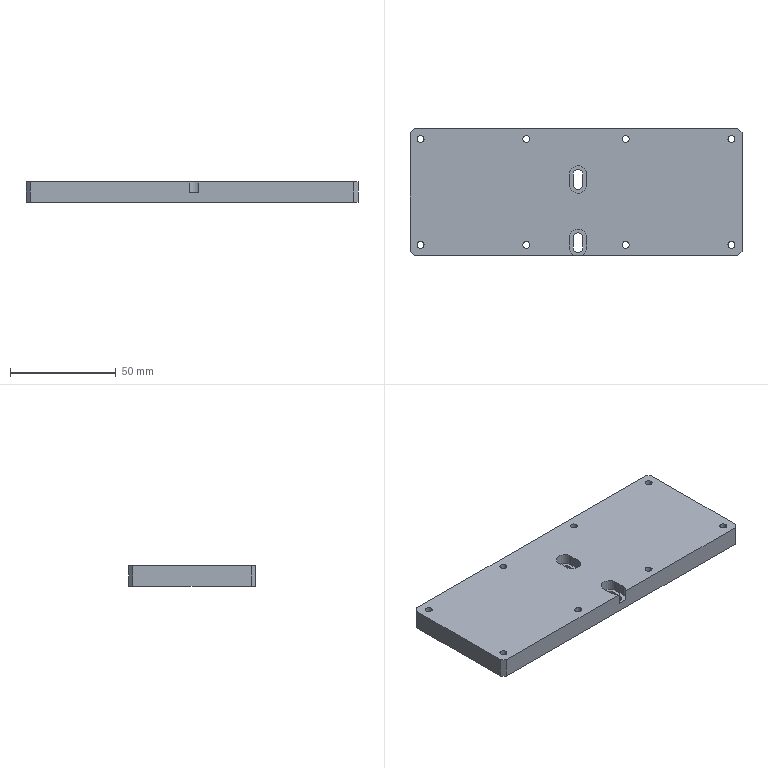Part | STEP file | 05-02-02 adjustment platform base plate | 1 solid | 45 faces | box 157 x 60 x 9.5 mm | volume 87518 mm3 | cylinder 25 | plane 20 | commonest cylinder face diameters 3.3 x16 8 x5 4.5 x4
STEP:
#1=CARTESIAN_POINT('',(71.85,25.,0.));
#2=VERTEX_POINT('',#1);
#3=CARTESIAN_POINT('',(75.15,25.,0.));
#4=VERTEX_POINT('',#3);
#5=CARTESIAN_POINT('',(73.5,25.,0.));
#6=DIRECTION('',(0.,0.,1.));
#7=DIRECTION('',(1.,0.,0.));
#8=AXIS2_PLACEMENT_3D('',#5,#6,#7);
#9=CIRCLE('',#8,1.65);
#10=EDGE_CURVE('',#2,#4,#9,.T.);
#11=ORIENTED_EDGE('',*,*,#10,.F.);
#12=CARTESIAN_POINT('',(71.85,25.,9.5));
#13=VERTEX_POINT('',#12);
#14=CARTESIAN_POINT('',(71.85,25.,9.5));
#15=DIRECTION('',(0.,0.,1.));
#16=VECTOR('',#15,1000.);
#17=LINE('',#14,#16);
#18=EDGE_CURVE('',#2,#13,#17,.T.);
#19=ORIENTED_EDGE('',*,*,#18,.T.);
#20=CARTESIAN_POINT('',(75.15,25.,9.5));
#21=VERTEX_POINT('',#20);
#22=CARTESIAN_POINT('',(73.5,25.,9.5));
#23=DIRECTION('',(0.,0.,1.));
#24=DIRECTION('',(1.,0.,0.));
#25=AXIS2_PLACEMENT_3D('',#22,#23,#24);
#26=CIRCLE('',#25,1.65);
#27=EDGE_CURVE('',#13,#21,#26,.T.);
#28=ORIENTED_EDGE('',*,*,#27,.T.);
#29=CARTESIAN_POINT('',(75.15,25.,9.5));
#30=DIRECTION('',(0.,0.,1.));
#31=VECTOR('',#30,1000.);
#32=LINE('',#29,#31);
#33=EDGE_CURVE('',#4,#21,#32,.T.);
#34=ORIENTED_EDGE('',*,*,#33,.F.);
#35=EDGE_LOOP('',(#11,#19,#28,#34));
#36=FACE_OUTER_BOUND('',#35,.T.);
#37=CARTESIAN_POINT('',(73.5,25.,9.5));
#38=DIRECTION('',(0.,0.,1.));
#39=DIRECTION('',(1.,0.,0.));
#40=AXIS2_PLACEMENT_3D('',#37,#38,#39);
#41=CYLINDRICAL_SURFACE('',#40,1.65);
#42=ADVANCED_FACE('',(#36),#41,.F.);
#43=CARTESIAN_POINT('',(21.85,-25.,0.));
#44=VERTEX_POINT('',#43);
#45=CARTESIAN_POINT('',(25.15,-25.,0.));
#46=VERTEX_POINT('',#45);
#47=CARTESIAN_POINT('',(23.5,-25.,0.));
#48=DIRECTION('',(0.,0.,1.));
#49=DIRECTION('',(1.,0.,0.));
#50=AXIS2_PLACEMENT_3D('',#47,#48,#49);
#51=CIRCLE('',#50,1.65);
#52=EDGE_CURVE('',#44,#46,#51,.T.);
#53=ORIENTED_EDGE('',*,*,#52,.F.);
#54=CARTESIAN_POINT('',(21.85,-25.,9.5));
#55=VERTEX_POINT('',#54);
#56=CARTESIAN_POINT('',(21.85,-25.,9.5));
#57=DIRECTION('',(0.,0.,1.));
#58=VECTOR('',#57,1000.);
#59=LINE('',#56,#58);
#60=EDGE_CURVE('',#44,#55,#59,.T.);
#61=ORIENTED_EDGE('',*,*,#60,.T.);
#62=CARTESIAN_POINT('',(25.15,-25.,9.5));
#63=VERTEX_POINT('',#62);
#64=CARTESIAN_POINT('',(23.5,-25.,9.5));
#65=DIRECTION('',(0.,0.,1.));
#66=DIRECTION('',(1.,0.,0.));
#67=AXIS2_PLACEMENT_3D('',#64,#65,#66);
#68=CIRCLE('',#67,1.65);
#69=EDGE_CURVE('',#55,#63,#68,.T.);
#70=ORIENTED_EDGE('',*,*,#69,.T.);
#71=CARTESIAN_POINT('',(25.15,-25.,9.5));
#72=DIRECTION('',(0.,0.,1.));
#73=VECTOR('',#72,1000.);
#74=LINE('',#71,#73);
#75=EDGE_CURVE('',#46,#63,#74,.T.);
#76=ORIENTED_EDGE('',*,*,#75,.F.);
#77=EDGE_LOOP('',(#53,#61,#70,#76));
#78=FACE_OUTER_BOUND('',#77,.T.);
#79=CARTESIAN_POINT('',(23.5,-25.,9.5));
#80=DIRECTION('',(0.,0.,1.));
#81=DIRECTION('',(1.,0.,0.));
#82=AXIS2_PLACEMENT_3D('',#79,#80,#81);
#83=CYLINDRICAL_SURFACE('',#82,1.65);
#84=ADVANCED_FACE('',(#78),#83,.F.);
#85=CARTESIAN_POINT('',(71.85,-25.,0.));
#86=VERTEX_POINT('',#85);
#87=CARTESIAN_POINT('',(75.15,-25.,0.));
#88=VERTEX_POINT('',#87);
#89=CARTESIAN_POINT('',(73.5,-25.,0.));
#90=DIRECTION('',(0.,0.,1.));
#91=DIRECTION('',(1.,0.,0.));
#92=AXIS2_PLACEMENT_3D('',#89,#90,#91);
#93=CIRCLE('',#92,1.65);
#94=EDGE_CURVE('',#86,#88,#93,.T.);
#95=ORIENTED_EDGE('',*,*,#94,.F.);
#96=CARTESIAN_POINT('',(71.85,-25.,9.5));
#97=VERTEX_POINT('',#96);
#98=CARTESIAN_POINT('',(71.85,-25.,9.5));
#99=DIRECTION('',(0.,0.,1.));
#100=VECTOR('',#99,1000.);
#101=LINE('',#98,#100);
#102=EDGE_CURVE('',#86,#97,#101,.T.);
#103=ORIENTED_EDGE('',*,*,#102,.T.);
#104=CARTESIAN_POINT('',(75.15,-25.,9.5));
#105=VERTEX_POINT('',#104);
#106=CARTESIAN_POINT('',(73.5,-25.,9.5));
#107=DIRECTION('',(0.,0.,1.));
#108=DIRECTION('',(1.,0.,0.));
#109=AXIS2_PLACEMENT_3D('',#106,#107,#108);
#110=CIRCLE('',#109,1.65);
#111=EDGE_CURVE('',#97,#105,#110,.T.);
#112=ORIENTED_EDGE('',*,*,#111,.T.);
#113=CARTESIAN_POINT('',(75.15,-25.,9.5));
#114=DIRECTION('',(0.,0.,1.));
#115=VECTOR('',#114,1000.);
#116=LINE('',#113,#115);
#117=EDGE_CURVE('',#88,#105,#116,.T.);
#118=ORIENTED_EDGE('',*,*,#117,.F.);
#119=EDGE_LOOP('',(#95,#103,#112,#118));
#120=FACE_OUTER_BOUND('',#119,.T.);
#121=CARTESIAN_POINT('',(73.5,-25.,9.5));
#122=DIRECTION('',(0.,0.,1.));
#123=DIRECTION('',(1.,0.,0.));
#124=AXIS2_PLACEMENT_3D('',#121,#122,#123);
#125=CYLINDRICAL_SURFACE('',#124,1.65);
#126=ADVANCED_FACE('',(#120),#125,.F.);
#127=CARTESIAN_POINT('',(21.85,25.,0.));
#128=VERTEX_POINT('',#127);
#129=CARTESIAN_POINT('',(25.15,25.,0.));
#130=VERTEX_POINT('',#129);
#131=CARTESIAN_POINT('',(23.5,25.,0.));
#132=DIRECTION('',(0.,0.,1.));
#133=DIRECTION('',(1.,0.,0.));
#134=AXIS2_PLACEMENT_3D('',#131,#132,#133);
#135=CIRCLE('',#134,1.65);
#136=EDGE_CURVE('',#128,#130,#135,.T.);
#137=ORIENTED_EDGE('',*,*,#136,.F.);
#138=CARTESIAN_POINT('',(21.85,25.,9.5));
#139=VERTEX_POINT('',#138);
#140=CARTESIAN_POINT('',(21.85,25.,9.5));
#141=DIRECTION('',(0.,0.,1.));
#142=VECTOR('',#141,1000.);
#143=LINE('',#140,#142);
#144=EDGE_CURVE('',#128,#139,#143,.T.);
#145=ORIENTED_EDGE('',*,*,#144,.T.);
#146=CARTESIAN_POINT('',(25.15,25.,9.5));
#147=VERTEX_POINT('',#146);
#148=CARTESIAN_POINT('',(23.5,25.,9.5));
#149=DIRECTION('',(0.,0.,1.));
#150=DIRECTION('',(1.,0.,0.));
#151=AXIS2_PLACEMENT_3D('',#148,#149,#150);
#152=CIRCLE('',#151,1.65);
#153=EDGE_CURVE('',#139,#147,#152,.T.);
#154=ORIENTED_EDGE('',*,*,#153,.T.);
#155=CARTESIAN_POINT('',(25.15,25.,9.5));
#156=DIRECTION('',(0.,0.,1.));
#157=VECTOR('',#156,1000.);
#158=LINE('',#155,#157);
#159=EDGE_CURVE('',#130,#147,#158,.T.);
#160=ORIENTED_EDGE('',*,*,#159,.F.);
#161=EDGE_LOOP('',(#137,#145,#154,#160));
#162=FACE_OUTER_BOUND('',#161,.T.);
#163=CARTESIAN_POINT('',(23.5,25.,9.5));
#164=DIRECTION('',(0.,0.,1.));
#165=DIRECTION('',(1.,0.,0.));
#166=AXIS2_PLACEMENT_3D('',#163,#164,#165);
#167=CYLINDRICAL_SURFACE('',#166,1.65);
#168=ADVANCED_FACE('',(#162),#167,.F.);
#169=CARTESIAN_POINT('',(-75.15,25.,0.));
#170=VERTEX_POINT('',#169);
#171=CARTESIAN_POINT('',(-71.85,25.,0.));
#172=VERTEX_POINT('',#171);
#173=CARTESIAN_POINT('',(-73.5,25.,0.));
#174=DIRECTION('',(0.,0.,1.));
#175=DIRECTION('',(1.,0.,0.));
#176=AXIS2_PLACEMENT_3D('',#173,#174,#175);
#177=CIRCLE('',#176,1.65);
#178=EDGE_CURVE('',#170,#172,#177,.T.);
#179=ORIENTED_EDGE('',*,*,#178,.F.);
#180=CARTESIAN_POINT('',(-75.15,25.,9.5));
#181=VERTEX_POINT('',#180);
#182=CARTESIAN_POINT('',(-75.15,25.,9.5));
#183=DIRECTION('',(0.,0.,1.));
#184=VECTOR('',#183,1000.);
#185=LINE('',#182,#184);
#186=EDGE_CURVE('',#170,#181,#185,.T.);
#187=ORIENTED_EDGE('',*,*,#186,.T.);
#188=CARTESIAN_POINT('',(-71.85,25.,9.5));
#189=VERTEX_POINT('',#188);
#190=CARTESIAN_POINT('',(-73.5,25.,9.5));
#191=DIRECTION('',(0.,0.,1.));
#192=DIRECTION('',(1.,0.,0.));
#193=AXIS2_PLACEMENT_3D('',#190,#191,#192);
#194=CIRCLE('',#193,1.65);
#195=EDGE_CURVE('',#181,#189,#194,.T.);
#196=ORIENTED_EDGE('',*,*,#195,.T.);
#197=CARTESIAN_POINT('',(-71.85,25.,9.5));
#198=DIRECTION('',(0.,0.,1.));
#199=VECTOR('',#198,1000.);
#200=LINE('',#197,#199);
#201=EDGE_CURVE('',#172,#189,#200,.T.);
#202=ORIENTED_EDGE('',*,*,#201,.F.);
#203=EDGE_LOOP('',(#179,#187,#196,#202));
#204=FACE_OUTER_BOUND('',#203,.T.);
#205=CARTESIAN_POINT('',(-73.5,25.,9.5));
#206=DIRECTION('',(0.,0.,1.));
#207=DIRECTION('',(1.,0.,0.));
#208=AXIS2_PLACEMENT_3D('',#205,#206,#207);
#209=CYLINDRICAL_SURFACE('',#208,1.65);
#210=ADVANCED_FACE('',(#204),#209,.F.);
#211=CARTESIAN_POINT('',(-25.15,25.,0.));
#212=VERTEX_POINT('',#211);
#213=CARTESIAN_POINT('',(-21.85,25.,0.));
#214=VERTEX_POINT('',#213);
#215=CARTESIAN_POINT('',(-23.5,25.,0.));
#216=DIRECTION('',(0.,0.,1.));
#217=DIRECTION('',(1.,0.,0.));
#218=AXIS2_PLACEMENT_3D('',#215,#216,#217);
#219=CIRCLE('',#218,1.65);
#220=EDGE_CURVE('',#212,#214,#219,.T.);
#221=ORIENTED_EDGE('',*,*,#220,.F.);
#222=CARTESIAN_POINT('',(-25.15,25.,9.5));
#223=VERTEX_POINT('',#222);
#224=CARTESIAN_POINT('',(-25.15,25.,9.5));
#225=DIRECTION('',(0.,0.,1.));
#226=VECTOR('',#225,1000.);
#227=LINE('',#224,#226);
#228=EDGE_CURVE('',#212,#223,#227,.T.);
#229=ORIENTED_EDGE('',*,*,#228,.T.);
#230=CARTESIAN_POINT('',(-21.85,25.,9.5));
#231=VERTEX_POINT('',#230);
#232=CARTESIAN_POINT('',(-23.5,25.,9.5));
#233=DIRECTION('',(0.,0.,1.));
#234=DIRECTION('',(1.,0.,0.));
#235=AXIS2_PLACEMENT_3D('',#232,#233,#234);
#236=CIRCLE('',#235,1.65);
#237=EDGE_CURVE('',#223,#231,#236,.T.);
#238=ORIENTED_EDGE('',*,*,#237,.T.);
#239=CARTESIAN_POINT('',(-21.85,25.,9.5));
#240=DIRECTION('',(0.,0.,1.));
#241=VECTOR('',#240,1000.);
#242=LINE('',#239,#241);
#243=EDGE_CURVE('',#214,#231,#242,.T.);
#244=ORIENTED_EDGE('',*,*,#243,.F.);
#245=EDGE_LOOP('',(#221,#229,#238,#244));
#246=FACE_OUTER_BOUND('',#245,.T.);
#247=CARTESIAN_POINT('',(-23.5,25.,9.5));
#248=DIRECTION('',(0.,0.,1.));
#249=DIRECTION('',(1.,0.,0.));
#250=AXIS2_PLACEMENT_3D('',#247,#248,#249);
#251=CYLINDRICAL_SURFACE('',#250,1.65);
#252=ADVANCED_FACE('',(#246),#251,.F.);
#253=CARTESIAN_POINT('',(-75.15,-25.,0.));
#254=VERTEX_POINT('',#253);
#255=CARTESIAN_POINT('',(-71.85,-25.,0.));
#256=VERTEX_POINT('',#255);
#257=CARTESIAN_POINT('',(-73.5,-25.,0.));
#258=DIRECTION('',(0.,0.,1.));
#259=DIRECTION('',(1.,0.,0.));
#260=AXIS2_PLACEMENT_3D('',#257,#258,#259);
#261=CIRCLE('',#260,1.65);
#262=EDGE_CURVE('',#254,#256,#261,.T.);
#263=ORIENTED_EDGE('',*,*,#262,.F.);
#264=CARTESIAN_POINT('',(-75.15,-25.,9.5));
#265=VERTEX_POINT('',#264);
#266=CARTESIAN_POINT('',(-75.15,-25.,9.5));
#267=DIRECTION('',(0.,0.,1.));
#268=VECTOR('',#267,1000.);
#269=LINE('',#266,#268);
#270=EDGE_CURVE('',#254,#265,#269,.T.);
#271=ORIENTED_EDGE('',*,*,#270,.T.);
#272=CARTESIAN_POINT('',(-71.85,-25.,9.5));
#273=VERTEX_POINT('',#272);
#274=CARTESIAN_POINT('',(-73.5,-25.,9.5));
#275=DIRECTION('',(0.,0.,1.));
#276=DIRECTION('',(1.,0.,0.));
#277=AXIS2_PLACEMENT_3D('',#274,#275,#276);
#278=CIRCLE('',#277,1.65);
#279=EDGE_CURVE('',#265,#273,#278,.T.);
#280=ORIENTED_EDGE('',*,*,#279,.T.);
#281=CARTESIAN_POINT('',(-71.85,-25.,9.5));
#282=DIRECTION('',(0.,0.,1.));
#283=VECTOR('',#282,1000.);
#284=LINE('',#281,#283);
#285=EDGE_CURVE('',#256,#273,#284,.T.);
#286=ORIENTED_EDGE('',*,*,#285,.F.);
#287=EDGE_LOOP('',(#263,#271,#280,#286));
#288=FACE_OUTER_BOUND('',#287,.T.);
#289=CARTESIAN_POINT('',(-73.5,-25.,9.5));
#290=DIRECTION('',(0.,0.,1.));
#291=DIRECTION('',(1.,0.,0.));
#292=AXIS2_PLACEMENT_3D('',#289,#290,#291);
#293=CYLINDRICAL_SURFACE('',#292,1.65);
#294=ADVANCED_FACE('',(#288),#293,.F.);
#295=CARTESIAN_POINT('',(-25.15,-25.,0.));
#296=VERTEX_POINT('',#295);
#297=CARTESIAN_POINT('',(-21.85,-25.,0.));
#298=VERTEX_POINT('',#297);
#299=CARTESIAN_POINT('',(-23.5,-25.,0.));
#300=DIRECTION('',(0.,0.,1.));
#301=DIRECTION('',(1.,0.,0.));
#302=AXIS2_PLACEMENT_3D('',#299,#300,#301);
#303=CIRCLE('',#302,1.65);
#304=EDGE_CURVE('',#296,#298,#303,.T.);
#305=ORIENTED_EDGE('',*,*,#304,.F.);
#306=CARTESIAN_POINT('',(-25.15,-25.,9.5));
#307=VERTEX_POINT('',#306);
#308=CARTESIAN_POINT('',(-25.15,-25.,9.5));
#309=DIRECTION('',(0.,0.,1.));
#310=VECTOR('',#309,1000.);
#311=LINE('',#308,#310);
#312=EDGE_CURVE('',#296,#307,#311,.T.);
#313=ORIENTED_EDGE('',*,*,#312,.T.);
#314=CARTESIAN_POINT('',(-21.85,-25.,9.5));
#315=VERTEX_POINT('',#314);
#316=CARTESIAN_POINT('',(-23.5,-25.,9.5));
#317=DIRECTION('',(0.,0.,1.));
#318=DIRECTION('',(1.,0.,0.));
#319=AXIS2_PLACEMENT_3D('',#316,#317,#318);
#320=CIRCLE('',#319,1.65);
#321=EDGE_CURVE('',#307,#315,#320,.T.);
#322=ORIENTED_EDGE('',*,*,#321,.T.);
#323=CARTESIAN_POINT('',(-21.85,-25.,9.5));
#324=DIRECTION('',(0.,0.,1.));
#325=VECTOR('',#324,1000.);
#326=LINE('',#323,#325);
#327=EDGE_CURVE('',#298,#315,#326,.T.);
#328=ORIENTED_EDGE('',*,*,#327,.F.);
#329=EDGE_LOOP('',(#305,#313,#322,#328));
#330=FACE_OUTER_BOUND('',#329,.T.);
#331=CARTESIAN_POINT('',(-23.5,-25.,9.5));
#332=DIRECTION('',(0.,0.,1.));
#333=DIRECTION('',(1.,0.,0.));
#334=AXIS2_PLACEMENT_3D('',#331,#332,#333);
#335=CYLINDRICAL_SURFACE('',#334,1.65);
#336=ADVANCED_FACE('',(#330),#335,.F.);
#337=CARTESIAN_POINT('',(-1.25,-21.5,4.5));
#338=VERTEX_POINT('',#337);
#339=CARTESIAN_POINT('',(3.25,-21.5,4.5));
#340=VERTEX_POINT('',#339);
#341=CARTESIAN_POINT('',(1.,-21.5,4.5));
#342=DIRECTION('',(0.,0.,-1.));
#343=DIRECTION('',(1.,0.,0.));
#344=AXIS2_PLACEMENT_3D('',#341,#342,#343);
#345=CIRCLE('',#344,2.25);
#346=EDGE_CURVE('',#338,#340,#345,.T.);
#347=ORIENTED_EDGE('',*,*,#346,.F.);
#348=CARTESIAN_POINT('',(-1.25,-21.5,0.));
#349=VERTEX_POINT('',#348);
#350=CARTESIAN_POINT('',(-1.25,-21.5,-0.5));
#351=DIRECTION('',(0.,0.,1.));
#352=VECTOR('',#351,1000.);
#353=LINE('',#350,#352);
#354=EDGE_CURVE('',#349,#338,#353,.T.);
#355=ORIENTED_EDGE('',*,*,#354,.F.);
#356=CARTESIAN_POINT('',(3.25,-21.5,0.));
#357=VERTEX_POINT('',#356);
#358=CARTESIAN_POINT('',(1.,-21.5,0.));
#359=DIRECTION('',(0.,0.,1.));
#360=DIRECTION('',(1.,0.,0.));
#361=AXIS2_PLACEMENT_3D('',#358,#359,#360);
#362=CIRCLE('',#361,2.25);
#363=EDGE_CURVE('',#357,#349,#362,.T.);
#364=ORIENTED_EDGE('',*,*,#363,.F.);
#365=CARTESIAN_POINT('',(3.25,-21.5,-0.5));
#366=DIRECTION('',(0.,0.,1.));
#367=VECTOR('',#366,1000.);
#368=LINE('',#365,#367);
#369=EDGE_CURVE('',#357,#340,#368,.T.);
#370=ORIENTED_EDGE('',*,*,#369,.T.);
#371=EDGE_LOOP('',(#347,#355,#364,#370));
#372=FACE_OUTER_BOUND('',#371,.T.);
#373=CARTESIAN_POINT('',(1.,-21.5,-0.5));
#374=DIRECTION('',(0.,0.,1.));
#375=DIRECTION('',(1.,0.,0.));
#376=AXIS2_PLACEMENT_3D('',#373,#374,#375);
#377=CYLINDRICAL_SURFACE('',#376,2.25);
#378=ADVANCED_FACE('',(#372),#377,.F.);
#379=CARTESIAN_POINT('',(3.25,-26.5,4.5));
#380=VERTEX_POINT('',#379);
#381=CARTESIAN_POINT('',(3.25,-21.5,4.5));
#382=DIRECTION('',(0.,-1.,0.));
#383=VECTOR('',#382,1000.);
#384=LINE('',#381,#383);
#385=EDGE_CURVE('',#340,#380,#384,.T.);
#386=ORIENTED_EDGE('',*,*,#385,.F.);
#387=ORIENTED_EDGE('',*,*,#369,.F.);
#388=CARTESIAN_POINT('',(3.25,-26.5,0.));
#389=VERTEX_POINT('',#388);
#390=CARTESIAN_POINT('',(3.25,-30.,0.));
#391=DIRECTION('',(0.,1.,0.));
#392=VECTOR('',#391,1000.);
#393=LINE('',#390,#392);
#394=EDGE_CURVE('',#389,#357,#393,.T.);
#395=ORIENTED_EDGE('',*,*,#394,.F.);
#396=CARTESIAN_POINT('',(3.25,-26.5,-0.5));
#397=DIRECTION('',(0.,0.,1.));
#398=VECTOR('',#397,1000.);
#399=LINE('',#396,#398);
#400=EDGE_CURVE('',#389,#380,#399,.T.);
#401=ORIENTED_EDGE('',*,*,#400,.T.);
#402=EDGE_LOOP('',(#386,#387,#395,#401));
#403=FACE_OUTER_BOUND('',#402,.T.);
#404=CARTESIAN_POINT('',(3.25,-21.5,-0.5));
#405=DIRECTION('',(1.,0.,0.));
#406=DIRECTION('',(0.,1.,0.));
#407=AXIS2_PLACEMENT_3D('',#404,#405,#406);
#408=PLANE('',#407);
#409=ADVANCED_FACE('',(#403),#408,.F.);
#410=CARTESIAN_POINT('',(-1.25,-26.5,4.5));
#411=VERTEX_POINT('',#410);
#412=CARTESIAN_POINT('',(1.,-26.5,4.5));
#413=DIRECTION('',(0.,0.,-1.));
#414=DIRECTION('',(1.,0.,0.));
#415=AXIS2_PLACEMENT_3D('',#412,#413,#414);
#416=CIRCLE('',#415,2.25);
#417=EDGE_CURVE('',#380,#411,#416,.T.);
#418=ORIENTED_EDGE('',*,*,#417,.F.);
#419=ORIENTED_EDGE('',*,*,#400,.F.);
#420=CARTESIAN_POINT('',(-1.25,-26.5,0.));
#421=VERTEX_POINT('',#420);
#422=CARTESIAN_POINT('',(1.,-26.5,0.));
#423=DIRECTION('',(0.,0.,1.));
#424=DIRECTION('',(1.,0.,0.));
#425=AXIS2_PLACEMENT_3D('',#422,#423,#424);
#426=CIRCLE('',#425,2.25);
#427=EDGE_CURVE('',#421,#389,#426,.T.);
#428=ORIENTED_EDGE('',*,*,#427,.F.);
#429=CARTESIAN_POINT('',(-1.25,-26.5,-0.5));
#430=DIRECTION('',(0.,0.,1.));
#431=VECTOR('',#430,1000.);
#432=LINE('',#429,#431);
#433=EDGE_CURVE('',#421,#411,#432,.T.);
#434=ORIENTED_EDGE('',*,*,#433,.T.);
#435=EDGE_LOOP('',(#418,#419,#428,#434));
#436=FACE_OUTER_BOUND('',#435,.T.);
#437=CARTESIAN_POINT('',(1.,-26.5,-0.5));
#438=DIRECTION('',(0.,0.,1.));
#439=DIRECTION('',(1.,0.,0.));
#440=AXIS2_PLACEMENT_3D('',#437,#438,#439);
#441=CYLINDRICAL_SURFACE('',#440,2.25);
#442=ADVANCED_FACE('',(#436),#441,.F.);
#443=CARTESIAN_POINT('',(-1.25,-21.5,4.5));
#444=DIRECTION('',(0.,1.,0.));
#445=VECTOR('',#444,1000.);
#446=LINE('',#443,#445);
#447=EDGE_CURVE('',#411,#338,#446,.T.);
#448=ORIENTED_EDGE('',*,*,#447,.F.);
#449=ORIENTED_EDGE('',*,*,#433,.F.);
#450=CARTESIAN_POINT('',(-1.25,-30.,0.));
#451=DIRECTION('',(0.,-1.,0.));
#452=VECTOR('',#451,1000.);
#453=LINE('',#450,#452);
#454=EDGE_CURVE('',#349,#421,#453,.T.);
#455=ORIENTED_EDGE('',*,*,#454,.F.);
#456=ORIENTED_EDGE('',*,*,#354,.T.);
#457=EDGE_LOOP('',(#448,#449,#455,#456));
#458=FACE_OUTER_BOUND('',#457,.T.);
#459=CARTESIAN_POINT('',(-1.25,-21.5,-0.5));
#460=DIRECTION('',(-1.,0.,0.));
#461=DIRECTION('',(0.,-1.,0.));
#462=AXIS2_PLACEMENT_3D('',#459,#460,#461);
#463=PLANE('',#462);
#464=ADVANCED_FACE('',(#458),#463,.F.);
#465=CARTESIAN_POINT('',(-1.25,8.5,4.5));
#466=VERTEX_POINT('',#465);
#467=CARTESIAN_POINT('',(3.25,8.5,4.5));
#468=VERTEX_POINT('',#467);
#469=CARTESIAN_POINT('',(1.,8.5,4.5));
#470=DIRECTION('',(0.,0.,-1.));
#471=DIRECTION('',(1.,0.,0.));
#472=AXIS2_PLACEMENT_3D('',#469,#470,#471);
#473=CIRCLE('',#472,2.25);
#474=EDGE_CURVE('',#466,#468,#473,.T.);
#475=ORIENTED_EDGE('',*,*,#474,.F.);
#476=CARTESIAN_POINT('',(-1.25,8.5,0.));
#477=VERTEX_POINT('',#476);
#478=CARTESIAN_POINT('',(-1.25,8.5,-0.5));
#479=DIRECTION('',(0.,0.,1.));
#480=VECTOR('',#479,1000.);
#481=LINE('',#478,#480);
#482=EDGE_CURVE('',#477,#466,#481,.T.);
#483=ORIENTED_EDGE('',*,*,#482,.F.);
#484=CARTESIAN_POINT('',(3.25,8.5,0.));
#485=VERTEX_POINT('',#484);
#486=CARTESIAN_POINT('',(1.,8.5,0.));
#487=DIRECTION('',(0.,0.,1.));
#488=DIRECTION('',(1.,0.,0.));
#489=AXIS2_PLACEMENT_3D('',#486,#487,#488);
#490=CIRCLE('',#489,2.25);
#491=EDGE_CURVE('',#485,#477,#490,.T.);
#492=ORIENTED_EDGE('',*,*,#491,.F.);
#493=CARTESIAN_POINT('',(3.25,8.5,-0.5));
#494=DIRECTION('',(0.,0.,1.));
#495=VECTOR('',#494,1000.);
#496=LINE('',#493,#495);
#497=EDGE_CURVE('',#485,#468,#496,.T.);
#498=ORIENTED_EDGE('',*,*,#497,.T.);
#499=EDGE_LOOP('',(#475,#483,#492,#498));
#500=FACE_OUTER_BOUND('',#499,.T.);
#501=CARTESIAN_POINT('',(1.,8.5,-0.5));
#502=DIRECTION('',(0.,0.,1.));
#503=DIRECTION('',(1.,0.,0.));
#504=AXIS2_PLACEMENT_3D('',#501,#502,#503);
#505=CYLINDRICAL_SURFACE('',#504,2.25);
#506=ADVANCED_FACE('',(#500),#505,.F.);
#507=CARTESIAN_POINT('',(3.25,3.5,4.5));
#508=VERTEX_POINT('',#507);
#509=CARTESIAN_POINT('',(3.25,8.5,4.5));
#510=DIRECTION('',(0.,-1.,0.));
#511=VECTOR('',#510,1000.);
#512=LINE('',#509,#511);
#513=EDGE_CURVE('',#468,#508,#512,.T.);
#514=ORIENTED_EDGE('',*,*,#513,.F.);
#515=ORIENTED_EDGE('',*,*,#497,.F.);
#516=CARTESIAN_POINT('',(3.25,3.5,0.));
#517=VERTEX_POINT('',#516);
#518=CARTESIAN_POINT('',(3.25,-30.,0.));
#519=DIRECTION('',(0.,1.,0.));
#520=VECTOR('',#519,1000.);
#521=LINE('',#518,#520);
#522=EDGE_CURVE('',#517,#485,#521,.T.);
#523=ORIENTED_EDGE('',*,*,#522,.F.);
#524=CARTESIAN_POINT('',(3.25,3.5,-0.5));
#525=DIRECTION('',(0.,0.,1.));
#526=VECTOR('',#525,1000.);
#527=LINE('',#524,#526);
#528=EDGE_CURVE('',#517,#508,#527,.T.);
#529=ORIENTED_EDGE('',*,*,#528,.T.);
#530=EDGE_LOOP('',(#514,#515,#523,#529));
#531=FACE_OUTER_BOUND('',#530,.T.);
#532=CARTESIAN_POINT('',(3.25,8.5,-0.5));
#533=DIRECTION('',(1.,0.,0.));
#534=DIRECTION('',(0.,1.,0.));
#535=AXIS2_PLACEMENT_3D('',#532,#533,#534);
#536=PLANE('',#535);
#537=ADVANCED_FACE('',(#531),#536,.F.);
#538=CARTESIAN_POINT('',(-1.25,3.5,4.5));
#539=VERTEX_POINT('',#538);
#540=CARTESIAN_POINT('',(1.,3.5,4.5));
#541=DIRECTION('',(0.,0.,-1.));
#542=DIRECTION('',(1.,0.,0.));
#543=AXIS2_PLACEMENT_3D('',#540,#541,#542);
#544=CIRCLE('',#543,2.25);
#545=EDGE_CURVE('',#508,#539,#544,.T.);
#546=ORIENTED_EDGE('',*,*,#545,.F.);
#547=ORIENTED_EDGE('',*,*,#528,.F.);
#548=CARTESIAN_POINT('',(-1.25,3.5,0.));
#549=VERTEX_POINT('',#548);
#550=CARTESIAN_POINT('',(1.,3.5,0.));
#551=DIRECTION('',(0.,0.,1.));
#552=DIRECTION('',(1.,0.,0.));
#553=AXIS2_PLACEMENT_3D('',#550,#551,#552);
#554=CIRCLE('',#553,2.25);
#555=EDGE_CURVE('',#549,#517,#554,.T.);
#556=ORIENTED_EDGE('',*,*,#555,.F.);
#557=CARTESIAN_POINT('',(-1.25,3.5,-0.5));
#558=DIRECTION('',(0.,0.,1.));
#559=VECTOR('',#558,1000.);
#560=LINE('',#557,#559);
#561=EDGE_CURVE('',#549,#539,#560,.T.);
#562=ORIENTED_EDGE('',*,*,#561,.T.);
#563=EDGE_LOOP('',(#546,#547,#556,#562));
#564=FACE_OUTER_BOUND('',#563,.T.);
#565=CARTESIAN_POINT('',(1.,3.5,-0.5));
#566=DIRECTION('',(0.,0.,1.));
#567=DIRECTION('',(1.,0.,0.));
#568=AXIS2_PLACEMENT_3D('',#565,#566,#567);
#569=CYLINDRICAL_SURFACE('',#568,2.25);
#570=ADVANCED_FACE('',(#564),#569,.F.);
#571=CARTESIAN_POINT('',(-1.25,8.5,4.5));
#572=DIRECTION('',(0.,1.,0.));
#573=VECTOR('',#572,1000.);
#574=LINE('',#571,#573);
#575=EDGE_CURVE('',#539,#466,#574,.T.);
#576=ORIENTED_EDGE('',*,*,#575,.F.);
#577=ORIENTED_EDGE('',*,*,#561,.F.);
#578=CARTESIAN_POINT('',(-1.25,-30.,0.));
#579=DIRECTION('',(0.,-1.,0.));
#580=VECTOR('',#579,1000.);
#581=LINE('',#578,#580);
#582=EDGE_CURVE('',#477,#549,#581,.T.);
#583=ORIENTED_EDGE('',*,*,#582,.F.);
#584=ORIENTED_EDGE('',*,*,#482,.T.);
#585=EDGE_LOOP('',(#576,#577,#583,#584));
#586=FACE_OUTER_BOUND('',#585,.T.);
#587=CARTESIAN_POINT('',(-1.25,8.5,-0.5));
#588=DIRECTION('',(-1.,0.,0.));
#589=DIRECTION('',(0.,-1.,0.));
#590=AXIS2_PLACEMENT_3D('',#587,#588,#589);
#591=PLANE('',#590);
#592=ADVANCED_FACE('',(#586),#591,.F.);
#593=CARTESIAN_POINT('',(78.5,-28.,0.));
#594=VERTEX_POINT('',#593);
#595=CARTESIAN_POINT('',(78.5,28.,0.));
#596=VERTEX_POINT('',#595);
#597=CARTESIAN_POINT('',(78.5,30.,0.));
#598=DIRECTION('',(0.,1.,0.));
#599=VECTOR('',#598,1000.);
#600=LINE('',#597,#599);
#601=EDGE_CURVE('',#594,#596,#600,.T.);
#602=ORIENTED_EDGE('',*,*,#601,.T.);
#603=CARTESIAN_POINT('',(78.5,28.,9.5));
#604=VERTEX_POINT('',#603);
#605=CARTESIAN_POINT('',(78.5,28.,9.5));
#606=DIRECTION('',(0.,0.,1.));
#607=VECTOR('',#606,1000.);
#608=LINE('',#605,#607);
#609=EDGE_CURVE('',#596,#604,#608,.T.);
#610=ORIENTED_EDGE('',*,*,#609,.T.);
#611=CARTESIAN_POINT('',(78.5,-28.,9.5));
#612=VERTEX_POINT('',#611);
#613=CARTESIAN_POINT('',(78.5,30.,9.5));
#614=DIRECTION('',(0.,1.,0.));
#615=VECTOR('',#614,1000.);
#616=LINE('',#613,#615);
#617=EDGE_CURVE('',#612,#604,#616,.T.);
#618=ORIENTED_EDGE('',*,*,#617,.F.);
#619=CARTESIAN_POINT('',(78.5,-28.,9.5));
#620=DIRECTION('',(0.,0.,-1.));
#621=VECTOR('',#620,1000.);
#622=LINE('',#619,#621);
#623=EDGE_CURVE('',#612,#594,#622,.T.);
#624=ORIENTED_EDGE('',*,*,#623,.T.);
#625=EDGE_LOOP('',(#602,#610,#618,#624));
#626=FACE_OUTER_BOUND('',#625,.T.);
#627=CARTESIAN_POINT('',(78.5,30.,9.5));
#628=DIRECTION('',(-1.,0.,0.));
#629=DIRECTION('',(0.,-1.,0.));
#630=AXIS2_PLACEMENT_3D('',#627,#628,#629);
#631=PLANE('',#630);
#632=ADVANCED_FACE('',(#626),#631,.F.);
#633=CARTESIAN_POINT('',(76.5,30.,9.5));
#634=VERTEX_POINT('',#633);
#635=CARTESIAN_POINT('',(-76.5,30.,9.5));
#636=VERTEX_POINT('',#635);
#637=CARTESIAN_POINT('',(-78.5,30.,9.5));
#638=DIRECTION('',(-1.,0.,0.));
#639=VECTOR('',#638,1000.);
#640=LINE('',#637,#639);
#641=EDGE_CURVE('',#634,#636,#640,.T.);
#642=ORIENTED_EDGE('',*,*,#641,.F.);
#643=CARTESIAN_POINT('',(76.5,30.,0.));
#644=VERTEX_POINT('',#643);
#645=CARTESIAN_POINT('',(76.5,30.,9.5));
#646=DIRECTION('',(0.,0.,-1.));
#647=VECTOR('',#646,1000.);
#648=LINE('',#645,#647);
#649=EDGE_CURVE('',#634,#644,#648,.T.);
#650=ORIENTED_EDGE('',*,*,#649,.T.);
#651=CARTESIAN_POINT('',(-76.5,30.,0.));
#652=VERTEX_POINT('',#651);
#653=CARTESIAN_POINT('',(-78.5,30.,0.));
#654=DIRECTION('',(-1.,0.,0.));
#655=VECTOR('',#654,1000.);
#656=LINE('',#653,#655);
#657=EDGE_CURVE('',#644,#652,#656,.T.);
#658=ORIENTED_EDGE('',*,*,#657,.T.);
#659=CARTESIAN_POINT('',(-76.5,30.,9.5));
#660=DIRECTION('',(0.,0.,1.));
#661=VECTOR('',#660,1000.);
#662=LINE('',#659,#661);
#663=EDGE_CURVE('',#652,#636,#662,.T.);
#664=ORIENTED_EDGE('',*,*,#663,.T.);
#665=EDGE_LOOP('',(#642,#650,#658,#664));
#666=FACE_OUTER_BOUND('',#665,.T.);
#667=CARTESIAN_POINT('',(-78.5,30.,9.5));
#668=DIRECTION('',(0.,-1.,0.));
#669=DIRECTION('',(0.,0.,-1.));
#670=AXIS2_PLACEMENT_3D('',#667,#668,#669);
#671=PLANE('',#670);
#672=ADVANCED_FACE('',(#666),#671,.F.);
#673=CARTESIAN_POINT('',(-78.5,28.,0.));
#674=VERTEX_POINT('',#673);
#675=CARTESIAN_POINT('',(-78.5,-28.,0.));
#676=VERTEX_POINT('',#675);
#677=CARTESIAN_POINT('',(-78.5,30.,0.));
#678=DIRECTION('',(0.,-1.,0.));
#679=VECTOR('',#678,1000.);
#680=LINE('',#677,#679);
#681=EDGE_CURVE('',#674,#676,#680,.T.);
#682=ORIENTED_EDGE('',*,*,#681,.T.);
#683=CARTESIAN_POINT('',(-78.5,-28.,9.5));
#684=VERTEX_POINT('',#683);
#685=CARTESIAN_POINT('',(-78.5,-28.,9.5));
#686=DIRECTION('',(0.,0.,1.));
#687=VECTOR('',#686,1000.);
#688=LINE('',#685,#687);
#689=EDGE_CURVE('',#676,#684,#688,.T.);
#690=ORIENTED_EDGE('',*,*,#689,.T.);
#691=CARTESIAN_POINT('',(-78.5,28.,9.5));
#692=VERTEX_POINT('',#691);
#693=CARTESIAN_POINT('',(-78.5,30.,9.5));
#694=DIRECTION('',(0.,-1.,0.));
#695=VECTOR('',#694,1000.);
#696=LINE('',#693,#695);
#697=EDGE_CURVE('',#692,#684,#696,.T.);
#698=ORIENTED_EDGE('',*,*,#697,.F.);
#699=CARTESIAN_POINT('',(-78.5,28.,9.5));
#700=DIRECTION('',(0.,0.,-1.));
#701=VECTOR('',#700,1000.);
#702=LINE('',#699,#701);
#703=EDGE_CURVE('',#692,#674,#702,.T.);
#704=ORIENTED_EDGE('',*,*,#703,.T.);
#705=EDGE_LOOP('',(#682,#690,#698,#704));
#706=FACE_OUTER_BOUND('',#705,.T.);
#707=CARTESIAN_POINT('',(-78.5,30.,9.5));
#708=DIRECTION('',(1.,0.,0.));
#709=DIRECTION('',(0.,1.,0.));
#710=AXIS2_PLACEMENT_3D('',#707,#708,#709);
#711=PLANE('',#710);
#712=ADVANCED_FACE('',(#706),#711,.F.);
#713=CARTESIAN_POINT('',(-76.5,-30.,0.));
#714=VERTEX_POINT('',#713);
#715=CARTESIAN_POINT('',(76.5,-30.,0.));
#716=VERTEX_POINT('',#715);
#717=CARTESIAN_POINT('',(-78.5,-30.,0.));
#718=DIRECTION('',(1.,0.,0.));
#719=VECTOR('',#718,1000.);
#720=LINE('',#717,#719);
#721=EDGE_CURVE('',#714,#716,#720,.T.);
#722=ORIENTED_EDGE('',*,*,#721,.T.);
#723=CARTESIAN_POINT('',(76.5,-30.,9.5));
#724=VERTEX_POINT('',#723);
#725=CARTESIAN_POINT('',(76.5,-30.,9.5));
#726=DIRECTION('',(0.,0.,1.));
#727=VECTOR('',#726,1000.);
#728=LINE('',#725,#727);
#729=EDGE_CURVE('',#716,#724,#728,.T.);
#730=ORIENTED_EDGE('',*,*,#729,.T.);
#731=CARTESIAN_POINT('',(3.047,-30.,9.5));
#732=VERTEX_POINT('',#731);
#733=CARTESIAN_POINT('',(-78.5,-30.,9.5));
#734=DIRECTION('',(1.,0.,0.));
#735=VECTOR('',#734,1000.);
#736=LINE('',#733,#735);
#737=EDGE_CURVE('',#732,#724,#736,.T.);
#738=ORIENTED_EDGE('',*,*,#737,.F.);
#739=CARTESIAN_POINT('',(3.047,-30.,4.5));
#740=VERTEX_POINT('',#739);
#741=CARTESIAN_POINT('',(3.047,-30.,4.5));
#742=DIRECTION('',(0.,0.,-1.));
#743=VECTOR('',#742,1000.);
#744=LINE('',#741,#743);
#745=EDGE_CURVE('',#732,#740,#744,.T.);
#746=ORIENTED_EDGE('',*,*,#745,.T.);
#747=CARTESIAN_POINT('',(-1.047,-30.,4.5));
#748=VERTEX_POINT('',#747);
#749=CARTESIAN_POINT('',(-78.5,-30.,4.5));
#750=DIRECTION('',(1.,0.,0.));
#751=VECTOR('',#750,1000.);
#752=LINE('',#749,#751);
#753=EDGE_CURVE('',#748,#740,#752,.T.);
#754=ORIENTED_EDGE('',*,*,#753,.F.);
#755=CARTESIAN_POINT('',(-1.047,-30.,9.5));
#756=VERTEX_POINT('',#755);
#757=CARTESIAN_POINT('',(-1.047,-30.,4.5));
#758=DIRECTION('',(0.,0.,1.));
#759=VECTOR('',#758,1000.);
#760=LINE('',#757,#759);
#761=EDGE_CURVE('',#748,#756,#760,.T.);
#762=ORIENTED_EDGE('',*,*,#761,.T.);
#763=CARTESIAN_POINT('',(-76.5,-30.,9.5));
#764=VERTEX_POINT('',#763);
#765=CARTESIAN_POINT('',(-78.5,-30.,9.5));
#766=DIRECTION('',(1.,0.,0.));
#767=VECTOR('',#766,1000.);
#768=LINE('',#765,#767);
#769=EDGE_CURVE('',#764,#756,#768,.T.);
#770=ORIENTED_EDGE('',*,*,#769,.F.);
#771=CARTESIAN_POINT('',(-76.5,-30.,9.5));
#772=DIRECTION('',(0.,0.,-1.));
#773=VECTOR('',#772,1000.);
#774=LINE('',#771,#773);
#775=EDGE_CURVE('',#764,#714,#774,.T.);
#776=ORIENTED_EDGE('',*,*,#775,.T.);
#777=EDGE_LOOP('',(#722,#730,#738,#746,#754,#762,#770,#776));
#778=FACE_OUTER_BOUND('',#777,.T.);
#779=CARTESIAN_POINT('',(-78.5,-30.,9.5));
#780=DIRECTION('',(0.,1.,0.));
#781=DIRECTION('',(0.,0.,1.));
#782=AXIS2_PLACEMENT_3D('',#779,#780,#781);
#783=PLANE('',#782);
#784=ADVANCED_FACE('',(#778),#783,.F.);
#785=ORIENTED_EDGE('',*,*,#617,.T.);
#786=CARTESIAN_POINT('',(107.5,-1.,9.5));
#787=DIRECTION('',(-0.7071,0.7071,0.));
#788=VECTOR('',#787,1000.);
#789=LINE('',#786,#788);
#790=EDGE_CURVE('',#604,#634,#789,.T.);
#791=ORIENTED_EDGE('',*,*,#790,.T.);
#792=ORIENTED_EDGE('',*,*,#641,.T.);
#793=CARTESIAN_POINT('',(-29.,77.5,9.5));
#794=DIRECTION('',(-0.7071,-0.7071,0.));
#795=VECTOR('',#794,1000.);
#796=LINE('',#793,#795);
#797=EDGE_CURVE('',#636,#692,#796,.T.);
#798=ORIENTED_EDGE('',*,*,#797,.T.);
#799=ORIENTED_EDGE('',*,*,#697,.T.);
#800=CARTESIAN_POINT('',(1.,-107.5,9.5));
#801=DIRECTION('',(0.7071,-0.7071,0.));
#802=VECTOR('',#801,1000.);
#803=LINE('',#800,#802);
#804=EDGE_CURVE('',#684,#764,#803,.T.);
#805=ORIENTED_EDGE('',*,*,#804,.T.);
#806=ORIENTED_EDGE('',*,*,#769,.T.);
#807=CARTESIAN_POINT('',(-3.,-26.563,9.5));
#808=VERTEX_POINT('',#807);
#809=CARTESIAN_POINT('',(1.,-26.563,9.5));
#810=DIRECTION('',(0.,0.,1.));
#811=DIRECTION('',(1.,0.,0.));
#812=AXIS2_PLACEMENT_3D('',#809,#810,#811);
#813=CIRCLE('',#812,4.);
#814=EDGE_CURVE('',#808,#756,#813,.T.);
#815=ORIENTED_EDGE('',*,*,#814,.F.);
#816=CARTESIAN_POINT('',(-3.,-21.5,9.5));
#817=VERTEX_POINT('',#816);
#818=CARTESIAN_POINT('',(-3.,-21.5,9.5));
#819=DIRECTION('',(0.,-1.,0.));
#820=VECTOR('',#819,1000.);
#821=LINE('',#818,#820);
#822=EDGE_CURVE('',#817,#808,#821,.T.);
#823=ORIENTED_EDGE('',*,*,#822,.F.);
#824=CARTESIAN_POINT('',(5.,-21.5,9.5));
#825=VERTEX_POINT('',#824);
#826=CARTESIAN_POINT('',(1.,-21.5,9.5));
#827=DIRECTION('',(0.,0.,1.));
#828=DIRECTION('',(1.,0.,0.));
#829=AXIS2_PLACEMENT_3D('',#826,#827,#828);
#830=CIRCLE('',#829,4.);
#831=EDGE_CURVE('',#825,#817,#830,.T.);
#832=ORIENTED_EDGE('',*,*,#831,.F.);
#833=CARTESIAN_POINT('',(5.,-26.563,9.5));
#834=VERTEX_POINT('',#833);
#835=CARTESIAN_POINT('',(5.,-21.5,9.5));
#836=DIRECTION('',(0.,1.,0.));
#837=VECTOR('',#836,1000.);
#838=LINE('',#835,#837);
#839=EDGE_CURVE('',#834,#825,#838,.T.);
#840=ORIENTED_EDGE('',*,*,#839,.F.);
#841=CARTESIAN_POINT('',(1.,-26.563,9.5));
#842=DIRECTION('',(0.,0.,1.));
#843=DIRECTION('',(1.,0.,0.));
#844=AXIS2_PLACEMENT_3D('',#841,#842,#843);
#845=CIRCLE('',#844,4.);
#846=EDGE_CURVE('',#732,#834,#845,.T.);
#847=ORIENTED_EDGE('',*,*,#846,.F.);
#848=ORIENTED_EDGE('',*,*,#737,.T.);
#849=CARTESIAN_POINT('',(77.5,-29.,9.5));
#850=DIRECTION('',(0.7071,0.7071,0.));
#851=VECTOR('',#850,1000.);
#852=LINE('',#849,#851);
#853=EDGE_CURVE('',#724,#612,#852,.T.);
#854=ORIENTED_EDGE('',*,*,#853,.T.);
#855=EDGE_LOOP('',(#785,#791,#792,#798,#799,#805,#806,#815,#823,#832,#840,#847,#848,#854));
#856=FACE_OUTER_BOUND('',#855,.T.);
#857=CARTESIAN_POINT('',(5.,8.5,9.5));
#858=VERTEX_POINT('',#857);
#859=CARTESIAN_POINT('',(-3.,8.5,9.5));
#860=VERTEX_POINT('',#859);
#861=CARTESIAN_POINT('',(1.,8.5,9.5));
#862=DIRECTION('',(0.,0.,1.));
#863=DIRECTION('',(1.,0.,0.));
#864=AXIS2_PLACEMENT_3D('',#861,#862,#863);
#865=CIRCLE('',#864,4.);
#866=EDGE_CURVE('',#858,#860,#865,.T.);
#867=ORIENTED_EDGE('',*,*,#866,.F.);
#868=CARTESIAN_POINT('',(5.,3.437,9.5));
#869=VERTEX_POINT('',#868);
#870=CARTESIAN_POINT('',(5.,8.5,9.5));
#871=DIRECTION('',(0.,1.,0.));
#872=VECTOR('',#871,1000.);
#873=LINE('',#870,#872);
#874=EDGE_CURVE('',#869,#858,#873,.T.);
#875=ORIENTED_EDGE('',*,*,#874,.F.);
#876=CARTESIAN_POINT('',(-3.,3.437,9.5));
#877=VERTEX_POINT('',#876);
#878=CARTESIAN_POINT('',(1.,3.437,9.5));
#879=DIRECTION('',(0.,0.,1.));
#880=DIRECTION('',(1.,0.,0.));
#881=AXIS2_PLACEMENT_3D('',#878,#879,#880);
#882=CIRCLE('',#881,4.);
#883=EDGE_CURVE('',#877,#869,#882,.T.);
#884=ORIENTED_EDGE('',*,*,#883,.F.);
#885=CARTESIAN_POINT('',(-3.,8.5,9.5));
#886=DIRECTION('',(0.,-1.,0.));
#887=VECTOR('',#886,1000.);
#888=LINE('',#885,#887);
#889=EDGE_CURVE('',#860,#877,#888,.T.);
#890=ORIENTED_EDGE('',*,*,#889,.F.);
#891=EDGE_LOOP('',(#867,#875,#884,#890));
#892=FACE_BOUND('',#891,.T.);
#893=CARTESIAN_POINT('',(73.5,25.,9.5));
#894=DIRECTION('',(0.,0.,1.));
#895=DIRECTION('',(1.,0.,0.));
#896=AXIS2_PLACEMENT_3D('',#893,#894,#895);
#897=CIRCLE('',#896,1.65);
#898=EDGE_CURVE('',#21,#13,#897,.T.);
#899=ORIENTED_EDGE('',*,*,#898,.F.);
#900=ORIENTED_EDGE('',*,*,#27,.F.);
#901=EDGE_LOOP('',(#899,#900));
#902=FACE_BOUND('',#901,.T.);
#903=CARTESIAN_POINT('',(23.5,-25.,9.5));
#904=DIRECTION('',(0.,0.,1.));
#905=DIRECTION('',(1.,0.,0.));
#906=AXIS2_PLACEMENT_3D('',#903,#904,#905);
#907=CIRCLE('',#906,1.65);
#908=EDGE_CURVE('',#63,#55,#907,.T.);
#909=ORIENTED_EDGE('',*,*,#908,.F.);
#910=ORIENTED_EDGE('',*,*,#69,.F.);
#911=EDGE_LOOP('',(#909,#910));
#912=FACE_BOUND('',#911,.T.);
#913=CARTESIAN_POINT('',(73.5,-25.,9.5));
#914=DIRECTION('',(0.,0.,1.));
#915=DIRECTION('',(1.,0.,0.));
#916=AXIS2_PLACEMENT_3D('',#913,#914,#915);
#917=CIRCLE('',#916,1.65);
#918=EDGE_CURVE('',#105,#97,#917,.T.);
#919=ORIENTED_EDGE('',*,*,#918,.F.);
#920=ORIENTED_EDGE('',*,*,#111,.F.);
#921=EDGE_LOOP('',(#919,#920));
#922=FACE_BOUND('',#921,.T.);
#923=CARTESIAN_POINT('',(23.5,25.,9.5));
#924=DIRECTION('',(0.,0.,1.));
#925=DIRECTION('',(1.,0.,0.));
#926=AXIS2_PLACEMENT_3D('',#923,#924,#925);
#927=CIRCLE('',#926,1.65);
#928=EDGE_CURVE('',#147,#139,#927,.T.);
#929=ORIENTED_EDGE('',*,*,#928,.F.);
#930=ORIENTED_EDGE('',*,*,#153,.F.);
#931=EDGE_LOOP('',(#929,#930));
#932=FACE_BOUND('',#931,.T.);
#933=CARTESIAN_POINT('',(-73.5,25.,9.5));
#934=DIRECTION('',(0.,0.,1.));
#935=DIRECTION('',(1.,0.,0.));
#936=AXIS2_PLACEMENT_3D('',#933,#934,#935);
#937=CIRCLE('',#936,1.65);
#938=EDGE_CURVE('',#189,#181,#937,.T.);
#939=ORIENTED_EDGE('',*,*,#938,.F.);
#940=ORIENTED_EDGE('',*,*,#195,.F.);
#941=EDGE_LOOP('',(#939,#940));
#942=FACE_BOUND('',#941,.T.);
#943=CARTESIAN_POINT('',(-23.5,25.,9.5));
#944=DIRECTION('',(0.,0.,1.));
#945=DIRECTION('',(1.,0.,0.));
#946=AXIS2_PLACEMENT_3D('',#943,#944,#945);
#947=CIRCLE('',#946,1.65);
#948=EDGE_CURVE('',#231,#223,#947,.T.);
#949=ORIENTED_EDGE('',*,*,#948,.F.);
#950=ORIENTED_EDGE('',*,*,#237,.F.);
#951=EDGE_LOOP('',(#949,#950));
#952=FACE_BOUND('',#951,.T.);
#953=CARTESIAN_POINT('',(-73.5,-25.,9.5));
#954=DIRECTION('',(0.,0.,1.));
#955=DIRECTION('',(1.,0.,0.));
#956=AXIS2_PLACEMENT_3D('',#953,#954,#955);
#957=CIRCLE('',#956,1.65);
#958=EDGE_CURVE('',#273,#265,#957,.T.);
#959=ORIENTED_EDGE('',*,*,#958,.F.);
#960=ORIENTED_EDGE('',*,*,#279,.F.);
#961=EDGE_LOOP('',(#959,#960));
#962=FACE_BOUND('',#961,.T.);
#963=CARTESIAN_POINT('',(-23.5,-25.,9.5));
#964=DIRECTION('',(0.,0.,1.));
#965=DIRECTION('',(1.,0.,0.));
#966=AXIS2_PLACEMENT_3D('',#963,#964,#965);
#967=CIRCLE('',#966,1.65);
#968=EDGE_CURVE('',#315,#307,#967,.T.);
#969=ORIENTED_EDGE('',*,*,#968,.F.);
#970=ORIENTED_EDGE('',*,*,#321,.F.);
#971=EDGE_LOOP('',(#969,#970));
#972=FACE_BOUND('',#971,.T.);
#973=CARTESIAN_POINT('',(78.5,-30.,9.5));
#974=DIRECTION('',(0.,0.,1.));
#975=DIRECTION('',(1.,0.,0.));
#976=AXIS2_PLACEMENT_3D('',#973,#974,#975);
#977=PLANE('',#976);
#978=ADVANCED_FACE('',(#856,#892,#902,#912,#922,#932,#942,#952,#962,#972),#977,.T.);
#979=ORIENTED_EDGE('',*,*,#394,.T.);
#980=ORIENTED_EDGE('',*,*,#363,.T.);
#981=ORIENTED_EDGE('',*,*,#454,.T.);
#982=ORIENTED_EDGE('',*,*,#427,.T.);
#983=EDGE_LOOP('',(#979,#980,#981,#982));
#984=FACE_BOUND('',#983,.T.);
#985=ORIENTED_EDGE('',*,*,#522,.T.);
#986=ORIENTED_EDGE('',*,*,#491,.T.);
#987=ORIENTED_EDGE('',*,*,#582,.T.);
#988=ORIENTED_EDGE('',*,*,#555,.T.);
#989=EDGE_LOOP('',(#985,#986,#987,#988));
#990=FACE_BOUND('',#989,.T.);
#991=CARTESIAN_POINT('',(73.5,25.,0.));
#992=DIRECTION('',(0.,0.,1.));
#993=DIRECTION('',(1.,0.,0.));
#994=AXIS2_PLACEMENT_3D('',#991,#992,#993);
#995=CIRCLE('',#994,1.65);
#996=EDGE_CURVE('',#4,#2,#995,.T.);
#997=ORIENTED_EDGE('',*,*,#996,.T.);
#998=ORIENTED_EDGE('',*,*,#10,.T.);
#999=EDGE_LOOP('',(#997,#998));
#1000=FACE_BOUND('',#999,.T.);
#1001=CARTESIAN_POINT('',(23.5,-25.,0.));
#1002=DIRECTION('',(0.,0.,1.));
#1003=DIRECTION('',(1.,0.,0.));
#1004=AXIS2_PLACEMENT_3D('',#1001,#1002,#1003);
#1005=CIRCLE('',#1004,1.65);
#1006=EDGE_CURVE('',#46,#44,#1005,.T.);
#1007=ORIENTED_EDGE('',*,*,#1006,.T.);
#1008=ORIENTED_EDGE('',*,*,#52,.T.);
#1009=EDGE_LOOP('',(#1007,#1008));
#1010=FACE_BOUND('',#1009,.T.);
#1011=CARTESIAN_POINT('',(73.5,-25.,0.));
#1012=DIRECTION('',(0.,0.,1.));
#1013=DIRECTION('',(1.,0.,0.));
#1014=AXIS2_PLACEMENT_3D('',#1011,#1012,#1013);
#1015=CIRCLE('',#1014,1.65);
#1016=EDGE_CURVE('',#88,#86,#1015,.T.);
#1017=ORIENTED_EDGE('',*,*,#1016,.T.);
#1018=ORIENTED_EDGE('',*,*,#94,.T.);
#1019=EDGE_LOOP('',(#1017,#1018));
#1020=FACE_BOUND('',#1019,.T.);
#1021=CARTESIAN_POINT('',(23.5,25.,0.));
#1022=DIRECTION('',(0.,0.,1.));
#1023=DIRECTION('',(1.,0.,0.));
#1024=AXIS2_PLACEMENT_3D('',#1021,#1022,#1023);
#1025=CIRCLE('',#1024,1.65);
#1026=EDGE_CURVE('',#130,#128,#1025,.T.);
#1027=ORIENTED_EDGE('',*,*,#1026,.T.);
#1028=ORIENTED_EDGE('',*,*,#136,.T.);
#1029=EDGE_LOOP('',(#1027,#1028));
#1030=FACE_BOUND('',#1029,.T.);
#1031=CARTESIAN_POINT('',(-73.5,25.,0.));
#1032=DIRECTION('',(0.,0.,1.));
#1033=DIRECTION('',(1.,0.,0.));
#1034=AXIS2_PLACEMENT_3D('',#1031,#1032,#1033);
#1035=CIRCLE('',#1034,1.65);
#1036=EDGE_CURVE('',#172,#170,#1035,.T.);
#1037=ORIENTED_EDGE('',*,*,#1036,.T.);
#1038=ORIENTED_EDGE('',*,*,#178,.T.);
#1039=EDGE_LOOP('',(#1037,#1038));
#1040=FACE_BOUND('',#1039,.T.);
#1041=CARTESIAN_POINT('',(-23.5,25.,0.));
#1042=DIRECTION('',(0.,0.,1.));
#1043=DIRECTION('',(1.,0.,0.));
#1044=AXIS2_PLACEMENT_3D('',#1041,#1042,#1043);
#1045=CIRCLE('',#1044,1.65);
#1046=EDGE_CURVE('',#214,#212,#1045,.T.);
#1047=ORIENTED_EDGE('',*,*,#1046,.T.);
#1048=ORIENTED_EDGE('',*,*,#220,.T.);
#1049=EDGE_LOOP('',(#1047,#1048));
#1050=FACE_BOUND('',#1049,.T.);
#1051=CARTESIAN_POINT('',(-73.5,-25.,0.));
#1052=DIRECTION('',(0.,0.,1.));
#1053=DIRECTION('',(1.,0.,0.));
#1054=AXIS2_PLACEMENT_3D('',#1051,#1052,#1053);
#1055=CIRCLE('',#1054,1.65);
#1056=EDGE_CURVE('',#256,#254,#1055,.T.);
#1057=ORIENTED_EDGE('',*,*,#1056,.T.);
#1058=ORIENTED_EDGE('',*,*,#262,.T.);
#1059=EDGE_LOOP('',(#1057,#1058));
#1060=FACE_BOUND('',#1059,.T.);
#1061=CARTESIAN_POINT('',(-23.5,-25.,0.));
#1062=DIRECTION('',(0.,0.,1.));
#1063=DIRECTION('',(1.,0.,0.));
#1064=AXIS2_PLACEMENT_3D('',#1061,#1062,#1063);
#1065=CIRCLE('',#1064,1.65);
#1066=EDGE_CURVE('',#298,#296,#1065,.T.);
#1067=ORIENTED_EDGE('',*,*,#1066,.T.);
#1068=ORIENTED_EDGE('',*,*,#304,.T.);
#1069=EDGE_LOOP('',(#1067,#1068));
#1070=FACE_BOUND('',#1069,.T.);
#1071=ORIENTED_EDGE('',*,*,#657,.F.);
#1072=CARTESIAN_POINT('',(76.5,30.,0.));
#1073=DIRECTION('',(0.7071,-0.7071,0.));
#1074=VECTOR('',#1073,1000.);
#1075=LINE('',#1072,#1074);
#1076=EDGE_CURVE('',#644,#596,#1075,.T.);
#1077=ORIENTED_EDGE('',*,*,#1076,.T.);
#1078=ORIENTED_EDGE('',*,*,#601,.F.);
#1079=CARTESIAN_POINT('',(78.5,-28.,0.));
#1080=DIRECTION('',(-0.7071,-0.7071,0.));
#1081=VECTOR('',#1080,1000.);
#1082=LINE('',#1079,#1081);
#1083=EDGE_CURVE('',#594,#716,#1082,.T.);
#1084=ORIENTED_EDGE('',*,*,#1083,.T.);
#1085=ORIENTED_EDGE('',*,*,#721,.F.);
#1086=CARTESIAN_POINT('',(-76.5,-30.,0.));
#1087=DIRECTION('',(-0.7071,0.7071,0.));
#1088=VECTOR('',#1087,1000.);
#1089=LINE('',#1086,#1088);
#1090=EDGE_CURVE('',#714,#676,#1089,.T.);
#1091=ORIENTED_EDGE('',*,*,#1090,.T.);
#1092=ORIENTED_EDGE('',*,*,#681,.F.);
#1093=CARTESIAN_POINT('',(-78.5,28.,0.));
#1094=DIRECTION('',(0.7071,0.7071,0.));
#1095=VECTOR('',#1094,1000.);
#1096=LINE('',#1093,#1095);
#1097=EDGE_CURVE('',#674,#652,#1096,.T.);
#1098=ORIENTED_EDGE('',*,*,#1097,.T.);
#1099=EDGE_LOOP('',(#1071,#1077,#1078,#1084,#1085,#1091,#1092,#1098));
#1100=FACE_OUTER_BOUND('',#1099,.T.);
#1101=CARTESIAN_POINT('',(78.5,-30.,0.));
#1102=DIRECTION('',(0.,0.,1.));
#1103=DIRECTION('',(1.,0.,0.));
#1104=AXIS2_PLACEMENT_3D('',#1101,#1102,#1103);
#1105=PLANE('',#1104);
#1106=ADVANCED_FACE('',(#984,#990,#1000,#1010,#1020,#1030,#1040,#1050,#1060,#1070,#1100),#1105,.F.);
#1107=ORIENTED_EDGE('',*,*,#312,.F.);
#1108=ORIENTED_EDGE('',*,*,#1066,.F.);
#1109=ORIENTED_EDGE('',*,*,#327,.T.);
#1110=ORIENTED_EDGE('',*,*,#968,.T.);
#1111=EDGE_LOOP('',(#1107,#1108,#1109,#1110));
#1112=FACE_OUTER_BOUND('',#1111,.T.);
#1113=CARTESIAN_POINT('',(-23.5,-25.,9.5));
#1114=DIRECTION('',(0.,0.,1.));
#1115=DIRECTION('',(1.,0.,0.));
#1116=AXIS2_PLACEMENT_3D('',#1113,#1114,#1115);
#1117=CYLINDRICAL_SURFACE('',#1116,1.65);
#1118=ADVANCED_FACE('',(#1112),#1117,.F.);
#1119=ORIENTED_EDGE('',*,*,#270,.F.);
#1120=ORIENTED_EDGE('',*,*,#1056,.F.);
#1121=ORIENTED_EDGE('',*,*,#285,.T.);
#1122=ORIENTED_EDGE('',*,*,#958,.T.);
#1123=EDGE_LOOP('',(#1119,#1120,#1121,#1122));
#1124=FACE_OUTER_BOUND('',#1123,.T.);
#1125=CARTESIAN_POINT('',(-73.5,-25.,9.5));
#1126=DIRECTION('',(0.,0.,1.));
#1127=DIRECTION('',(1.,0.,0.));
#1128=AXIS2_PLACEMENT_3D('',#1125,#1126,#1127);
#1129=CYLINDRICAL_SURFACE('',#1128,1.65);
#1130=ADVANCED_FACE('',(#1124),#1129,.F.);
#1131=ORIENTED_EDGE('',*,*,#228,.F.);
#1132=ORIENTED_EDGE('',*,*,#1046,.F.);
#1133=ORIENTED_EDGE('',*,*,#243,.T.);
#1134=ORIENTED_EDGE('',*,*,#948,.T.);
#1135=EDGE_LOOP('',(#1131,#1132,#1133,#1134));
#1136=FACE_OUTER_BOUND('',#1135,.T.);
#1137=CARTESIAN_POINT('',(-23.5,25.,9.5));
#1138=DIRECTION('',(0.,0.,1.));
#1139=DIRECTION('',(1.,0.,0.));
#1140=AXIS2_PLACEMENT_3D('',#1137,#1138,#1139);
#1141=CYLINDRICAL_SURFACE('',#1140,1.65);
#1142=ADVANCED_FACE('',(#1136),#1141,.F.);
#1143=ORIENTED_EDGE('',*,*,#186,.F.);
#1144=ORIENTED_EDGE('',*,*,#1036,.F.);
#1145=ORIENTED_EDGE('',*,*,#201,.T.);
#1146=ORIENTED_EDGE('',*,*,#938,.T.);
#1147=EDGE_LOOP('',(#1143,#1144,#1145,#1146));
#1148=FACE_OUTER_BOUND('',#1147,.T.);
#1149=CARTESIAN_POINT('',(-73.5,25.,9.5));
#1150=DIRECTION('',(0.,0.,1.));
#1151=DIRECTION('',(1.,0.,0.));
#1152=AXIS2_PLACEMENT_3D('',#1149,#1150,#1151);
#1153=CYLINDRICAL_SURFACE('',#1152,1.65);
#1154=ADVANCED_FACE('',(#1148),#1153,.F.);
#1155=ORIENTED_EDGE('',*,*,#144,.F.);
#1156=ORIENTED_EDGE('',*,*,#1026,.F.);
#1157=ORIENTED_EDGE('',*,*,#159,.T.);
#1158=ORIENTED_EDGE('',*,*,#928,.T.);
#1159=EDGE_LOOP('',(#1155,#1156,#1157,#1158));
#1160=FACE_OUTER_BOUND('',#1159,.T.);
#1161=CARTESIAN_POINT('',(23.5,25.,9.5));
#1162=DIRECTION('',(0.,0.,1.));
#1163=DIRECTION('',(1.,0.,0.));
#1164=AXIS2_PLACEMENT_3D('',#1161,#1162,#1163);
#1165=CYLINDRICAL_SURFACE('',#1164,1.65);
#1166=ADVANCED_FACE('',(#1160),#1165,.F.);
#1167=ORIENTED_EDGE('',*,*,#102,.F.);
#1168=ORIENTED_EDGE('',*,*,#1016,.F.);
#1169=ORIENTED_EDGE('',*,*,#117,.T.);
#1170=ORIENTED_EDGE('',*,*,#918,.T.);
#1171=EDGE_LOOP('',(#1167,#1168,#1169,#1170));
#1172=FACE_OUTER_BOUND('',#1171,.T.);
#1173=CARTESIAN_POINT('',(73.5,-25.,9.5));
#1174=DIRECTION('',(0.,0.,1.));
#1175=DIRECTION('',(1.,0.,0.));
#1176=AXIS2_PLACEMENT_3D('',#1173,#1174,#1175);
#1177=CYLINDRICAL_SURFACE('',#1176,1.65);
#1178=ADVANCED_FACE('',(#1172),#1177,.F.);
#1179=ORIENTED_EDGE('',*,*,#60,.F.);
#1180=ORIENTED_EDGE('',*,*,#1006,.F.);
#1181=ORIENTED_EDGE('',*,*,#75,.T.);
#1182=ORIENTED_EDGE('',*,*,#908,.T.);
#1183=EDGE_LOOP('',(#1179,#1180,#1181,#1182));
#1184=FACE_OUTER_BOUND('',#1183,.T.);
#1185=CARTESIAN_POINT('',(23.5,-25.,9.5));
#1186=DIRECTION('',(0.,0.,1.));
#1187=DIRECTION('',(1.,0.,0.));
#1188=AXIS2_PLACEMENT_3D('',#1185,#1186,#1187);
#1189=CYLINDRICAL_SURFACE('',#1188,1.65);
#1190=ADVANCED_FACE('',(#1184),#1189,.F.);
#1191=ORIENTED_EDGE('',*,*,#18,.F.);
#1192=ORIENTED_EDGE('',*,*,#996,.F.);
#1193=ORIENTED_EDGE('',*,*,#33,.T.);
#1194=ORIENTED_EDGE('',*,*,#898,.T.);
#1195=EDGE_LOOP('',(#1191,#1192,#1193,#1194));
#1196=FACE_OUTER_BOUND('',#1195,.T.);
#1197=CARTESIAN_POINT('',(73.5,25.,9.5));
#1198=DIRECTION('',(0.,0.,1.));
#1199=DIRECTION('',(1.,0.,0.));
#1200=AXIS2_PLACEMENT_3D('',#1197,#1198,#1199);
#1201=CYLINDRICAL_SURFACE('',#1200,1.65);
#1202=ADVANCED_FACE('',(#1196),#1201,.F.);
#1203=CARTESIAN_POINT('',(5.,8.5,4.5));
#1204=VERTEX_POINT('',#1203);
#1205=CARTESIAN_POINT('',(-3.,8.5,4.5));
#1206=VERTEX_POINT('',#1205);
#1207=CARTESIAN_POINT('',(1.,8.5,4.5));
#1208=DIRECTION('',(0.,0.,1.));
#1209=DIRECTION('',(1.,0.,0.));
#1210=AXIS2_PLACEMENT_3D('',#1207,#1208,#1209);
#1211=CIRCLE('',#1210,4.);
#1212=EDGE_CURVE('',#1204,#1206,#1211,.T.);
#1213=ORIENTED_EDGE('',*,*,#1212,.T.);
#1214=CARTESIAN_POINT('',(-3.,3.437,4.5));
#1215=VERTEX_POINT('',#1214);
#1216=CARTESIAN_POINT('',(-3.,8.5,4.5));
#1217=DIRECTION('',(0.,-1.,0.));
#1218=VECTOR('',#1217,1000.);
#1219=LINE('',#1216,#1218);
#1220=EDGE_CURVE('',#1206,#1215,#1219,.T.);
#1221=ORIENTED_EDGE('',*,*,#1220,.T.);
#1222=CARTESIAN_POINT('',(5.,3.437,4.5));
#1223=VERTEX_POINT('',#1222);
#1224=CARTESIAN_POINT('',(1.,3.437,4.5));
#1225=DIRECTION('',(0.,0.,1.));
#1226=DIRECTION('',(1.,0.,0.));
#1227=AXIS2_PLACEMENT_3D('',#1224,#1225,#1226);
#1228=CIRCLE('',#1227,4.);
#1229=EDGE_CURVE('',#1215,#1223,#1228,.T.);
#1230=ORIENTED_EDGE('',*,*,#1229,.T.);
#1231=CARTESIAN_POINT('',(5.,8.5,4.5));
#1232=DIRECTION('',(0.,1.,0.));
#1233=VECTOR('',#1232,1000.);
#1234=LINE('',#1231,#1233);
#1235=EDGE_CURVE('',#1223,#1204,#1234,.T.);
#1236=ORIENTED_EDGE('',*,*,#1235,.T.);
#1237=EDGE_LOOP('',(#1213,#1221,#1230,#1236));
#1238=FACE_OUTER_BOUND('',#1237,.T.);
#1239=ORIENTED_EDGE('',*,*,#474,.T.);
#1240=ORIENTED_EDGE('',*,*,#513,.T.);
#1241=ORIENTED_EDGE('',*,*,#545,.T.);
#1242=ORIENTED_EDGE('',*,*,#575,.T.);
#1243=EDGE_LOOP('',(#1239,#1240,#1241,#1242));
#1244=FACE_BOUND('',#1243,.T.);
#1245=CARTESIAN_POINT('',(1.,8.5,4.5));
#1246=DIRECTION('',(0.,0.,1.));
#1247=DIRECTION('',(1.,0.,0.));
#1248=AXIS2_PLACEMENT_3D('',#1245,#1246,#1247);
#1249=PLANE('',#1248);
#1250=ADVANCED_FACE('',(#1238,#1244),#1249,.T.);
#1251=ORIENTED_EDGE('',*,*,#866,.T.);
#1252=CARTESIAN_POINT('',(-3.,8.5,4.5));
#1253=DIRECTION('',(0.,0.,1.));
#1254=VECTOR('',#1253,1000.);
#1255=LINE('',#1252,#1254);
#1256=EDGE_CURVE('',#1206,#860,#1255,.T.);
#1257=ORIENTED_EDGE('',*,*,#1256,.F.);
#1258=ORIENTED_EDGE('',*,*,#1212,.F.);
#1259=CARTESIAN_POINT('',(5.,8.5,4.5));
#1260=DIRECTION('',(0.,0.,1.));
#1261=VECTOR('',#1260,1000.);
#1262=LINE('',#1259,#1261);
#1263=EDGE_CURVE('',#1204,#858,#1262,.T.);
#1264=ORIENTED_EDGE('',*,*,#1263,.T.);
#1265=EDGE_LOOP('',(#1251,#1257,#1258,#1264));
#1266=FACE_OUTER_BOUND('',#1265,.T.);
#1267=CARTESIAN_POINT('',(1.,8.5,4.5));
#1268=DIRECTION('',(0.,0.,1.));
#1269=DIRECTION('',(1.,0.,0.));
#1270=AXIS2_PLACEMENT_3D('',#1267,#1268,#1269);
#1271=CYLINDRICAL_SURFACE('',#1270,4.);
#1272=ADVANCED_FACE('',(#1266),#1271,.F.);
#1273=ORIENTED_EDGE('',*,*,#874,.T.);
#1274=ORIENTED_EDGE('',*,*,#1263,.F.);
#1275=ORIENTED_EDGE('',*,*,#1235,.F.);
#1276=CARTESIAN_POINT('',(5.,3.437,4.5));
#1277=DIRECTION('',(0.,0.,1.));
#1278=VECTOR('',#1277,1000.);
#1279=LINE('',#1276,#1278);
#1280=EDGE_CURVE('',#1223,#869,#1279,.T.);
#1281=ORIENTED_EDGE('',*,*,#1280,.T.);
#1282=EDGE_LOOP('',(#1273,#1274,#1275,#1281));
#1283=FACE_OUTER_BOUND('',#1282,.T.);
#1284=CARTESIAN_POINT('',(5.,8.5,4.5));
#1285=DIRECTION('',(1.,0.,0.));
#1286=DIRECTION('',(0.,1.,0.));
#1287=AXIS2_PLACEMENT_3D('',#1284,#1285,#1286);
#1288=PLANE('',#1287);
#1289=ADVANCED_FACE('',(#1283),#1288,.F.);
#1290=ORIENTED_EDGE('',*,*,#883,.T.);
#1291=ORIENTED_EDGE('',*,*,#1280,.F.);
#1292=ORIENTED_EDGE('',*,*,#1229,.F.);
#1293=CARTESIAN_POINT('',(-3.,3.437,4.5));
#1294=DIRECTION('',(0.,0.,1.));
#1295=VECTOR('',#1294,1000.);
#1296=LINE('',#1293,#1295);
#1297=EDGE_CURVE('',#1215,#877,#1296,.T.);
#1298=ORIENTED_EDGE('',*,*,#1297,.T.);
#1299=EDGE_LOOP('',(#1290,#1291,#1292,#1298));
#1300=FACE_OUTER_BOUND('',#1299,.T.);
#1301=CARTESIAN_POINT('',(1.,3.437,4.5));
#1302=DIRECTION('',(0.,0.,1.));
#1303=DIRECTION('',(1.,0.,0.));
#1304=AXIS2_PLACEMENT_3D('',#1301,#1302,#1303);
#1305=CYLINDRICAL_SURFACE('',#1304,4.);
#1306=ADVANCED_FACE('',(#1300),#1305,.F.);
#1307=ORIENTED_EDGE('',*,*,#889,.T.);
#1308=ORIENTED_EDGE('',*,*,#1297,.F.);
#1309=ORIENTED_EDGE('',*,*,#1220,.F.);
#1310=ORIENTED_EDGE('',*,*,#1256,.T.);
#1311=EDGE_LOOP('',(#1307,#1308,#1309,#1310));
#1312=FACE_OUTER_BOUND('',#1311,.T.);
#1313=CARTESIAN_POINT('',(-3.,8.5,4.5));
#1314=DIRECTION('',(-1.,0.,0.));
#1315=DIRECTION('',(0.,-1.,0.));
#1316=AXIS2_PLACEMENT_3D('',#1313,#1314,#1315);
#1317=PLANE('',#1316);
#1318=ADVANCED_FACE('',(#1312),#1317,.F.);
#1319=CARTESIAN_POINT('',(-3.,-26.563,4.5));
#1320=VERTEX_POINT('',#1319);
#1321=CARTESIAN_POINT('',(1.,-26.563,4.5));
#1322=DIRECTION('',(0.,0.,1.));
#1323=DIRECTION('',(1.,0.,0.));
#1324=AXIS2_PLACEMENT_3D('',#1321,#1322,#1323);
#1325=CIRCLE('',#1324,4.);
#1326=EDGE_CURVE('',#1320,#748,#1325,.T.);
#1327=ORIENTED_EDGE('',*,*,#1326,.F.);
#1328=CARTESIAN_POINT('',(-3.,-26.563,4.5));
#1329=DIRECTION('',(0.,0.,1.));
#1330=VECTOR('',#1329,1000.);
#1331=LINE('',#1328,#1330);
#1332=EDGE_CURVE('',#1320,#808,#1331,.T.);
#1333=ORIENTED_EDGE('',*,*,#1332,.T.);
#1334=ORIENTED_EDGE('',*,*,#814,.T.);
#1335=ORIENTED_EDGE('',*,*,#761,.F.);
#1336=EDGE_LOOP('',(#1327,#1333,#1334,#1335));
#1337=FACE_OUTER_BOUND('',#1336,.T.);
#1338=CARTESIAN_POINT('',(1.,-26.563,4.5));
#1339=DIRECTION('',(0.,0.,1.));
#1340=DIRECTION('',(1.,0.,0.));
#1341=AXIS2_PLACEMENT_3D('',#1338,#1339,#1340);
#1342=CYLINDRICAL_SURFACE('',#1341,4.);
#1343=ADVANCED_FACE('',(#1337),#1342,.F.);
#1344=ORIENTED_EDGE('',*,*,#846,.T.);
#1345=CARTESIAN_POINT('',(5.,-26.563,4.5));
#1346=VERTEX_POINT('',#1345);
#1347=CARTESIAN_POINT('',(5.,-26.563,4.5));
#1348=DIRECTION('',(0.,0.,1.));
#1349=VECTOR('',#1348,1000.);
#1350=LINE('',#1347,#1349);
#1351=EDGE_CURVE('',#1346,#834,#1350,.T.);
#1352=ORIENTED_EDGE('',*,*,#1351,.F.);
#1353=CARTESIAN_POINT('',(1.,-26.563,4.5));
#1354=DIRECTION('',(0.,0.,1.));
#1355=DIRECTION('',(1.,0.,0.));
#1356=AXIS2_PLACEMENT_3D('',#1353,#1354,#1355);
#1357=CIRCLE('',#1356,4.);
#1358=EDGE_CURVE('',#740,#1346,#1357,.T.);
#1359=ORIENTED_EDGE('',*,*,#1358,.F.);
#1360=ORIENTED_EDGE('',*,*,#745,.F.);
#1361=EDGE_LOOP('',(#1344,#1352,#1359,#1360));
#1362=FACE_OUTER_BOUND('',#1361,.T.);
#1363=CARTESIAN_POINT('',(1.,-26.563,4.5));
#1364=DIRECTION('',(0.,0.,1.));
#1365=DIRECTION('',(1.,0.,0.));
#1366=AXIS2_PLACEMENT_3D('',#1363,#1364,#1365);
#1367=CYLINDRICAL_SURFACE('',#1366,4.);
#1368=ADVANCED_FACE('',(#1362),#1367,.F.);
#1369=ORIENTED_EDGE('',*,*,#346,.T.);
#1370=ORIENTED_EDGE('',*,*,#385,.T.);
#1371=ORIENTED_EDGE('',*,*,#417,.T.);
#1372=ORIENTED_EDGE('',*,*,#447,.T.);
#1373=EDGE_LOOP('',(#1369,#1370,#1371,#1372));
#1374=FACE_BOUND('',#1373,.T.);
#1375=ORIENTED_EDGE('',*,*,#753,.T.);
#1376=ORIENTED_EDGE('',*,*,#1358,.T.);
#1377=CARTESIAN_POINT('',(5.,-21.5,4.5));
#1378=VERTEX_POINT('',#1377);
#1379=CARTESIAN_POINT('',(5.,-21.5,4.5));
#1380=DIRECTION('',(0.,1.,0.));
#1381=VECTOR('',#1380,1000.);
#1382=LINE('',#1379,#1381);
#1383=EDGE_CURVE('',#1346,#1378,#1382,.T.);
#1384=ORIENTED_EDGE('',*,*,#1383,.T.);
#1385=CARTESIAN_POINT('',(-3.,-21.5,4.5));
#1386=VERTEX_POINT('',#1385);
#1387=CARTESIAN_POINT('',(1.,-21.5,4.5));
#1388=DIRECTION('',(0.,0.,1.));
#1389=DIRECTION('',(1.,0.,0.));
#1390=AXIS2_PLACEMENT_3D('',#1387,#1388,#1389);
#1391=CIRCLE('',#1390,4.);
#1392=EDGE_CURVE('',#1378,#1386,#1391,.T.);
#1393=ORIENTED_EDGE('',*,*,#1392,.T.);
#1394=CARTESIAN_POINT('',(-3.,-21.5,4.5));
#1395=DIRECTION('',(0.,-1.,0.));
#1396=VECTOR('',#1395,1000.);
#1397=LINE('',#1394,#1396);
#1398=EDGE_CURVE('',#1386,#1320,#1397,.T.);
#1399=ORIENTED_EDGE('',*,*,#1398,.T.);
#1400=ORIENTED_EDGE('',*,*,#1326,.T.);
#1401=EDGE_LOOP('',(#1375,#1376,#1384,#1393,#1399,#1400));
#1402=FACE_OUTER_BOUND('',#1401,.T.);
#1403=CARTESIAN_POINT('',(1.,-21.5,4.5));
#1404=DIRECTION('',(0.,0.,1.));
#1405=DIRECTION('',(1.,0.,0.));
#1406=AXIS2_PLACEMENT_3D('',#1403,#1404,#1405);
#1407=PLANE('',#1406);
#1408=ADVANCED_FACE('',(#1374,#1402),#1407,.T.);
#1409=ORIENTED_EDGE('',*,*,#831,.T.);
#1410=CARTESIAN_POINT('',(-3.,-21.5,4.5));
#1411=DIRECTION('',(0.,0.,1.));
#1412=VECTOR('',#1411,1000.);
#1413=LINE('',#1410,#1412);
#1414=EDGE_CURVE('',#1386,#817,#1413,.T.);
#1415=ORIENTED_EDGE('',*,*,#1414,.F.);
#1416=ORIENTED_EDGE('',*,*,#1392,.F.);
#1417=CARTESIAN_POINT('',(5.,-21.5,4.5));
#1418=DIRECTION('',(0.,0.,1.));
#1419=VECTOR('',#1418,1000.);
#1420=LINE('',#1417,#1419);
#1421=EDGE_CURVE('',#1378,#825,#1420,.T.);
#1422=ORIENTED_EDGE('',*,*,#1421,.T.);
#1423=EDGE_LOOP('',(#1409,#1415,#1416,#1422));
#1424=FACE_OUTER_BOUND('',#1423,.T.);
#1425=CARTESIAN_POINT('',(1.,-21.5,4.5));
#1426=DIRECTION('',(0.,0.,1.));
#1427=DIRECTION('',(1.,0.,0.));
#1428=AXIS2_PLACEMENT_3D('',#1425,#1426,#1427);
#1429=CYLINDRICAL_SURFACE('',#1428,4.);
#1430=ADVANCED_FACE('',(#1424),#1429,.F.);
#1431=ORIENTED_EDGE('',*,*,#839,.T.);
#1432=ORIENTED_EDGE('',*,*,#1421,.F.);
#1433=ORIENTED_EDGE('',*,*,#1383,.F.);
#1434=ORIENTED_EDGE('',*,*,#1351,.T.);
#1435=EDGE_LOOP('',(#1431,#1432,#1433,#1434));
#1436=FACE_OUTER_BOUND('',#1435,.T.);
#1437=CARTESIAN_POINT('',(5.,-21.5,4.5));
#1438=DIRECTION('',(1.,0.,0.));
#1439=DIRECTION('',(0.,1.,0.));
#1440=AXIS2_PLACEMENT_3D('',#1437,#1438,#1439);
#1441=PLANE('',#1440);
#1442=ADVANCED_FACE('',(#1436),#1441,.F.);
#1443=ORIENTED_EDGE('',*,*,#822,.T.);
#1444=ORIENTED_EDGE('',*,*,#1332,.F.);
#1445=ORIENTED_EDGE('',*,*,#1398,.F.);
#1446=ORIENTED_EDGE('',*,*,#1414,.T.);
#1447=EDGE_LOOP('',(#1443,#1444,#1445,#1446));
#1448=FACE_OUTER_BOUND('',#1447,.T.);
#1449=CARTESIAN_POINT('',(-3.,-21.5,4.5));
#1450=DIRECTION('',(-1.,0.,0.));
#1451=DIRECTION('',(0.,-1.,0.));
#1452=AXIS2_PLACEMENT_3D('',#1449,#1450,#1451);
#1453=PLANE('',#1452);
#1454=ADVANCED_FACE('',(#1448),#1453,.F.);
#1455=ORIENTED_EDGE('',*,*,#790,.F.);
#1456=ORIENTED_EDGE('',*,*,#609,.F.);
#1457=ORIENTED_EDGE('',*,*,#1076,.F.);
#1458=ORIENTED_EDGE('',*,*,#649,.F.);
#1459=EDGE_LOOP('',(#1455,#1456,#1457,#1458));
#1460=FACE_OUTER_BOUND('',#1459,.T.);
#1461=CARTESIAN_POINT('',(76.5,30.,9.5));
#1462=DIRECTION('',(-0.7071,-0.7071,0.));
#1463=DIRECTION('',(0.7071,-0.7071,0.));
#1464=AXIS2_PLACEMENT_3D('',#1461,#1462,#1463);
#1465=PLANE('',#1464);
#1466=ADVANCED_FACE('',(#1460),#1465,.F.);
#1467=ORIENTED_EDGE('',*,*,#853,.F.);
#1468=ORIENTED_EDGE('',*,*,#729,.F.);
#1469=ORIENTED_EDGE('',*,*,#1083,.F.);
#1470=ORIENTED_EDGE('',*,*,#623,.F.);
#1471=EDGE_LOOP('',(#1467,#1468,#1469,#1470));
#1472=FACE_OUTER_BOUND('',#1471,.T.);
#1473=CARTESIAN_POINT('',(78.5,-28.,9.5));
#1474=DIRECTION('',(-0.7071,0.7071,0.));
#1475=DIRECTION('',(-0.7071,-0.7071,0.));
#1476=AXIS2_PLACEMENT_3D('',#1473,#1474,#1475);
#1477=PLANE('',#1476);
#1478=ADVANCED_FACE('',(#1472),#1477,.F.);
#1479=ORIENTED_EDGE('',*,*,#804,.F.);
#1480=ORIENTED_EDGE('',*,*,#689,.F.);
#1481=ORIENTED_EDGE('',*,*,#1090,.F.);
#1482=ORIENTED_EDGE('',*,*,#775,.F.);
#1483=EDGE_LOOP('',(#1479,#1480,#1481,#1482));
#1484=FACE_OUTER_BOUND('',#1483,.T.);
#1485=CARTESIAN_POINT('',(-76.5,-30.,9.5));
#1486=DIRECTION('',(0.7071,0.7071,0.));
#1487=DIRECTION('',(-0.7071,0.7071,0.));
#1488=AXIS2_PLACEMENT_3D('',#1485,#1486,#1487);
#1489=PLANE('',#1488);
#1490=ADVANCED_FACE('',(#1484),#1489,.F.);
#1491=ORIENTED_EDGE('',*,*,#797,.F.);
#1492=ORIENTED_EDGE('',*,*,#663,.F.);
#1493=ORIENTED_EDGE('',*,*,#1097,.F.);
#1494=ORIENTED_EDGE('',*,*,#703,.F.);
#1495=EDGE_LOOP('',(#1491,#1492,#1493,#1494));
#1496=FACE_OUTER_BOUND('',#1495,.T.);
#1497=CARTESIAN_POINT('',(-78.5,28.,9.5));
#1498=DIRECTION('',(0.7071,-0.7071,0.));
#1499=DIRECTION('',(0.7071,0.7071,0.));
#1500=AXIS2_PLACEMENT_3D('',#1497,#1498,#1499);
#1501=PLANE('',#1500);
#1502=ADVANCED_FACE('',(#1496),#1501,.F.);
#1503=CLOSED_SHELL('',(#42,#84,#126,#168,#210,#252,#294,#336,#378,#409,#442,#464,#506,#537,#570,#592,#632,#672,#712,#784,#978,#1106,#1118,#1130,#1142,#1154,#1166,#1178,#1190,#1202,#1250,#1272,#1289,#1306,#1318,#1343,#1368,#1408,#1430,#1442,#1454,#1466,#1478,#1490,#1502));
#1504=MANIFOLD_SOLID_BREP('',#1503);
#1505=CARTESIAN_POINT('',(0.,0.,0.));
#1506=DIRECTION('',(0.,0.,1.));
#1507=DIRECTION('',(1.,0.,0.));
#1508=AXIS2_PLACEMENT_3D('',#1505,#1506,#1507);
#1509=(LENGTH_UNIT()NAMED_UNIT(*)SI_UNIT(.MILLI.,.METRE.));
#1510=UNCERTAINTY_MEASURE_WITH_UNIT(LENGTH_MEASURE(0.00001),#1509,'','');
#1511=(NAMED_UNIT(*)PLANE_ANGLE_UNIT()SI_UNIT($,.RADIAN.));
#1512=(NAMED_UNIT(*)SI_UNIT($,.STERADIAN.)SOLID_ANGLE_UNIT());
#1513=(GEOMETRIC_REPRESENTATION_CONTEXT(3)GLOBAL_UNCERTAINTY_ASSIGNED_CONTEXT((#1510))GLOBAL_UNIT_ASSIGNED_CONTEXT((#1509,#1511,#1512))REPRESENTATION_CONTEXT('',''));
#1514=ADVANCED_BREP_SHAPE_REPRESENTATION('',(#1504,#1508),#1513);